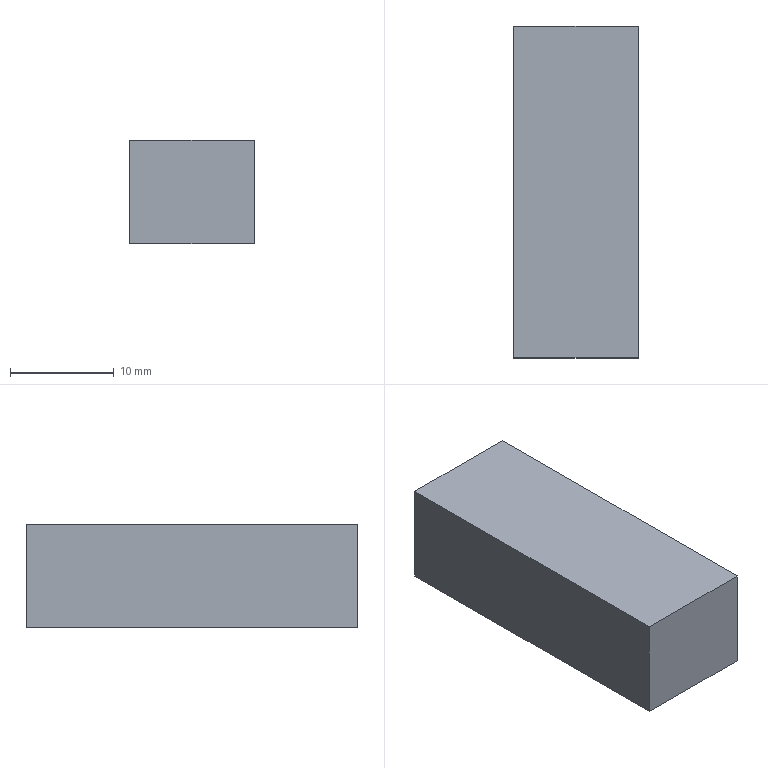Part | SolidWorks | features Extrusion 1 | 1 solid | 6 faces | box 12 x 32 x 10 mm | volume 3840 mm3 | plane 6
STEP:
#1=CARTESIAN_POINT('',(-6.,16.,5.));
#2=VERTEX_POINT('',#1);
#3=CARTESIAN_POINT('',(-6.,-16.,5.));
#4=VERTEX_POINT('',#3);
#5=CARTESIAN_POINT('',(-6.,16.,5.));
#6=DIRECTION('',(0.,-1.,0.));
#7=VECTOR('',#6,1000.);
#8=LINE('',#5,#7);
#9=EDGE_CURVE('',#2,#4,#8,.T.);
#10=ORIENTED_EDGE('',*,*,#9,.F.);
#11=CARTESIAN_POINT('',(-6.,16.,-5.));
#12=VERTEX_POINT('',#11);
#13=CARTESIAN_POINT('',(-6.,16.,-5.));
#14=DIRECTION('',(0.,0.,1.));
#15=VECTOR('',#14,1000.);
#16=LINE('',#13,#15);
#17=EDGE_CURVE('',#12,#2,#16,.T.);
#18=ORIENTED_EDGE('',*,*,#17,.F.);
#19=CARTESIAN_POINT('',(-6.,-16.,-5.));
#20=VERTEX_POINT('',#19);
#21=CARTESIAN_POINT('',(-6.,16.,-5.));
#22=DIRECTION('',(0.,-1.,0.));
#23=VECTOR('',#22,1000.);
#24=LINE('',#21,#23);
#25=EDGE_CURVE('',#12,#20,#24,.T.);
#26=ORIENTED_EDGE('',*,*,#25,.T.);
#27=CARTESIAN_POINT('',(-6.,-16.,-5.));
#28=DIRECTION('',(0.,0.,1.));
#29=VECTOR('',#28,1000.);
#30=LINE('',#27,#29);
#31=EDGE_CURVE('',#20,#4,#30,.T.);
#32=ORIENTED_EDGE('',*,*,#31,.T.);
#33=EDGE_LOOP('',(#10,#18,#26,#32));
#34=FACE_OUTER_BOUND('',#33,.T.);
#35=CARTESIAN_POINT('',(-6.,16.,-5.));
#36=DIRECTION('',(-1.,0.,0.));
#37=DIRECTION('',(0.,0.,1.));
#38=AXIS2_PLACEMENT_3D('',#35,#36,#37);
#39=PLANE('',#38);
#40=ADVANCED_FACE('',(#34),#39,.T.);
#41=CARTESIAN_POINT('',(6.,16.,5.));
#42=VERTEX_POINT('',#41);
#43=CARTESIAN_POINT('',(6.,16.,5.));
#44=DIRECTION('',(-1.,0.,0.));
#45=VECTOR('',#44,1000.);
#46=LINE('',#43,#45);
#47=EDGE_CURVE('',#42,#2,#46,.T.);
#48=ORIENTED_EDGE('',*,*,#47,.F.);
#49=CARTESIAN_POINT('',(6.,16.,-5.));
#50=VERTEX_POINT('',#49);
#51=CARTESIAN_POINT('',(6.,16.,-5.));
#52=DIRECTION('',(0.,0.,1.));
#53=VECTOR('',#52,1000.);
#54=LINE('',#51,#53);
#55=EDGE_CURVE('',#50,#42,#54,.T.);
#56=ORIENTED_EDGE('',*,*,#55,.F.);
#57=CARTESIAN_POINT('',(6.,16.,-5.));
#58=DIRECTION('',(-1.,0.,0.));
#59=VECTOR('',#58,1000.);
#60=LINE('',#57,#59);
#61=EDGE_CURVE('',#50,#12,#60,.T.);
#62=ORIENTED_EDGE('',*,*,#61,.T.);
#63=ORIENTED_EDGE('',*,*,#17,.T.);
#64=EDGE_LOOP('',(#48,#56,#62,#63));
#65=FACE_OUTER_BOUND('',#64,.T.);
#66=CARTESIAN_POINT('',(6.,16.,-5.));
#67=DIRECTION('',(0.,1.,0.));
#68=DIRECTION('',(0.,0.,1.));
#69=AXIS2_PLACEMENT_3D('',#66,#67,#68);
#70=PLANE('',#69);
#71=ADVANCED_FACE('',(#65),#70,.T.);
#72=CARTESIAN_POINT('',(6.,-16.,5.));
#73=VERTEX_POINT('',#72);
#74=CARTESIAN_POINT('',(6.,-16.,5.));
#75=DIRECTION('',(0.,1.,0.));
#76=VECTOR('',#75,1000.);
#77=LINE('',#74,#76);
#78=EDGE_CURVE('',#73,#42,#77,.T.);
#79=ORIENTED_EDGE('',*,*,#78,.F.);
#80=CARTESIAN_POINT('',(6.,-16.,-5.));
#81=VERTEX_POINT('',#80);
#82=CARTESIAN_POINT('',(6.,-16.,-5.));
#83=DIRECTION('',(0.,0.,1.));
#84=VECTOR('',#83,1000.);
#85=LINE('',#82,#84);
#86=EDGE_CURVE('',#81,#73,#85,.T.);
#87=ORIENTED_EDGE('',*,*,#86,.F.);
#88=CARTESIAN_POINT('',(6.,-16.,-5.));
#89=DIRECTION('',(0.,1.,0.));
#90=VECTOR('',#89,1000.);
#91=LINE('',#88,#90);
#92=EDGE_CURVE('',#81,#50,#91,.T.);
#93=ORIENTED_EDGE('',*,*,#92,.T.);
#94=ORIENTED_EDGE('',*,*,#55,.T.);
#95=EDGE_LOOP('',(#79,#87,#93,#94));
#96=FACE_OUTER_BOUND('',#95,.T.);
#97=CARTESIAN_POINT('',(6.,-16.,-5.));
#98=DIRECTION('',(1.,0.,0.));
#99=DIRECTION('',(0.,0.,-1.));
#100=AXIS2_PLACEMENT_3D('',#97,#98,#99);
#101=PLANE('',#100);
#102=ADVANCED_FACE('',(#96),#101,.T.);
#103=CARTESIAN_POINT('',(-6.,-16.,5.));
#104=DIRECTION('',(1.,0.,0.));
#105=VECTOR('',#104,1000.);
#106=LINE('',#103,#105);
#107=EDGE_CURVE('',#4,#73,#106,.T.);
#108=ORIENTED_EDGE('',*,*,#107,.F.);
#109=ORIENTED_EDGE('',*,*,#31,.F.);
#110=CARTESIAN_POINT('',(-6.,-16.,-5.));
#111=DIRECTION('',(1.,0.,0.));
#112=VECTOR('',#111,1000.);
#113=LINE('',#110,#112);
#114=EDGE_CURVE('',#20,#81,#113,.T.);
#115=ORIENTED_EDGE('',*,*,#114,.T.);
#116=ORIENTED_EDGE('',*,*,#86,.T.);
#117=EDGE_LOOP('',(#108,#109,#115,#116));
#118=FACE_OUTER_BOUND('',#117,.T.);
#119=CARTESIAN_POINT('',(-6.,-16.,-5.));
#120=DIRECTION('',(0.,-1.,0.));
#121=DIRECTION('',(0.,0.,-1.));
#122=AXIS2_PLACEMENT_3D('',#119,#120,#121);
#123=PLANE('',#122);
#124=ADVANCED_FACE('',(#118),#123,.T.);
#125=ORIENTED_EDGE('',*,*,#25,.F.);
#126=ORIENTED_EDGE('',*,*,#61,.F.);
#127=ORIENTED_EDGE('',*,*,#92,.F.);
#128=ORIENTED_EDGE('',*,*,#114,.F.);
#129=EDGE_LOOP('',(#125,#126,#127,#128));
#130=FACE_OUTER_BOUND('',#129,.T.);
#131=CARTESIAN_POINT('',(0.,0.,-5.));
#132=DIRECTION('',(0.,0.,1.));
#133=DIRECTION('',(1.,0.,0.));
#134=AXIS2_PLACEMENT_3D('',#131,#132,#133);
#135=PLANE('',#134);
#136=ADVANCED_FACE('',(#130),#135,.F.);
#137=ORIENTED_EDGE('',*,*,#9,.T.);
#138=ORIENTED_EDGE('',*,*,#107,.T.);
#139=ORIENTED_EDGE('',*,*,#78,.T.);
#140=ORIENTED_EDGE('',*,*,#47,.T.);
#141=EDGE_LOOP('',(#137,#138,#139,#140));
#142=FACE_OUTER_BOUND('',#141,.T.);
#143=CARTESIAN_POINT('',(0.,0.,5.));
#144=DIRECTION('',(0.,0.,1.));
#145=DIRECTION('',(1.,0.,0.));
#146=AXIS2_PLACEMENT_3D('',#143,#144,#145);
#147=PLANE('',#146);
#148=ADVANCED_FACE('',(#142),#147,.T.);
#149=CLOSED_SHELL('',(#40,#71,#102,#124,#136,#148));
#150=MANIFOLD_SOLID_BREP('',#149);
#151=CARTESIAN_POINT('',(0.,0.,0.));
#152=DIRECTION('',(0.,0.,1.));
#153=DIRECTION('',(1.,0.,0.));
#154=AXIS2_PLACEMENT_3D('',#151,#152,#153);
#155=(LENGTH_UNIT()NAMED_UNIT(*)SI_UNIT(.MILLI.,.METRE.));
#156=UNCERTAINTY_MEASURE_WITH_UNIT(LENGTH_MEASURE(0.00001),#155,'','');
#157=(NAMED_UNIT(*)PLANE_ANGLE_UNIT()SI_UNIT($,.RADIAN.));
#158=(NAMED_UNIT(*)SI_UNIT($,.STERADIAN.)SOLID_ANGLE_UNIT());
#159=(GEOMETRIC_REPRESENTATION_CONTEXT(3)GLOBAL_UNCERTAINTY_ASSIGNED_CONTEXT((#156))GLOBAL_UNIT_ASSIGNED_CONTEXT((#155,#157,#158))REPRESENTATION_CONTEXT('',''));
#160=ADVANCED_BREP_SHAPE_REPRESENTATION('',(#150,#154),#159);